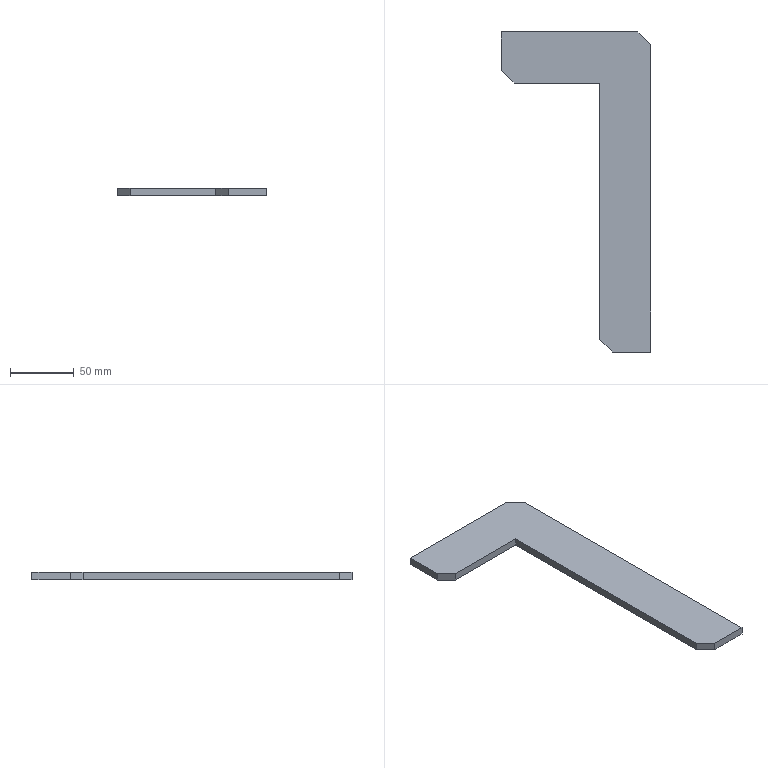Part | STEP file | X77-07102 | 1 solid | 11 faces | box 117 x 250.648 x 6 mm | volume 77736 mm3 | plane 11
STEP:
#1=CARTESIAN_POINT('',(-134.199,-59.214,0.));
#2=VERTEX_POINT('',#1);
#3=CARTESIAN_POINT('',(-241.199,-59.214,0.));
#4=VERTEX_POINT('',#3);
#5=CARTESIAN_POINT('',(-241.199,-59.214,0.));
#6=DIRECTION('',(-1.,0.,0.));
#7=VECTOR('',#6,1000.);
#8=LINE('',#5,#7);
#9=EDGE_CURVE('',#2,#4,#8,.T.);
#10=ORIENTED_EDGE('',*,*,#9,.T.);
#11=CARTESIAN_POINT('',(-241.199,-59.214,6.));
#12=VERTEX_POINT('',#11);
#13=CARTESIAN_POINT('',(-241.199,-59.214,6.));
#14=DIRECTION('',(0.,0.,-1.));
#15=VECTOR('',#14,1000.);
#16=LINE('',#13,#15);
#17=EDGE_CURVE('',#12,#4,#16,.T.);
#18=ORIENTED_EDGE('',*,*,#17,.F.);
#19=CARTESIAN_POINT('',(-134.199,-59.214,6.));
#20=VERTEX_POINT('',#19);
#21=CARTESIAN_POINT('',(-241.199,-59.214,6.));
#22=DIRECTION('',(-1.,0.,0.));
#23=VECTOR('',#22,1000.);
#24=LINE('',#21,#23);
#25=EDGE_CURVE('',#20,#12,#24,.T.);
#26=ORIENTED_EDGE('',*,*,#25,.F.);
#27=CARTESIAN_POINT('',(-134.199,-59.214,6.));
#28=DIRECTION('',(0.,0.,-1.));
#29=VECTOR('',#28,1000.);
#30=LINE('',#27,#29);
#31=EDGE_CURVE('',#20,#2,#30,.T.);
#32=ORIENTED_EDGE('',*,*,#31,.T.);
#33=EDGE_LOOP('',(#10,#18,#26,#32));
#34=FACE_OUTER_BOUND('',#33,.T.);
#35=CARTESIAN_POINT('',(-241.199,-59.214,6.));
#36=DIRECTION('',(0.,-1.,0.));
#37=DIRECTION('',(1.,0.,0.));
#38=AXIS2_PLACEMENT_3D('',#35,#36,#37);
#39=PLANE('',#38);
#40=ADVANCED_FACE('',(#34),#39,.F.);
#41=CARTESIAN_POINT('',(-241.199,-89.214,0.));
#42=VERTEX_POINT('',#41);
#43=CARTESIAN_POINT('',(-241.199,-59.214,0.));
#44=DIRECTION('',(0.,-1.,0.));
#45=VECTOR('',#44,1000.);
#46=LINE('',#43,#45);
#47=EDGE_CURVE('',#4,#42,#46,.T.);
#48=ORIENTED_EDGE('',*,*,#47,.T.);
#49=CARTESIAN_POINT('',(-241.199,-89.214,6.));
#50=VERTEX_POINT('',#49);
#51=CARTESIAN_POINT('',(-241.199,-89.214,6.));
#52=DIRECTION('',(0.,0.,1.));
#53=VECTOR('',#52,1000.);
#54=LINE('',#51,#53);
#55=EDGE_CURVE('',#42,#50,#54,.T.);
#56=ORIENTED_EDGE('',*,*,#55,.T.);
#57=CARTESIAN_POINT('',(-241.199,-59.214,6.));
#58=DIRECTION('',(0.,-1.,0.));
#59=VECTOR('',#58,1000.);
#60=LINE('',#57,#59);
#61=EDGE_CURVE('',#12,#50,#60,.T.);
#62=ORIENTED_EDGE('',*,*,#61,.F.);
#63=ORIENTED_EDGE('',*,*,#17,.T.);
#64=EDGE_LOOP('',(#48,#56,#62,#63));
#65=FACE_OUTER_BOUND('',#64,.T.);
#66=CARTESIAN_POINT('',(-241.199,-59.214,6.));
#67=DIRECTION('',(1.,0.,0.));
#68=DIRECTION('',(0.,1.,0.));
#69=AXIS2_PLACEMENT_3D('',#66,#67,#68);
#70=PLANE('',#69);
#71=ADVANCED_FACE('',(#65),#70,.F.);
#72=CARTESIAN_POINT('',(-231.199,-99.214,6.));
#73=VERTEX_POINT('',#72);
#74=CARTESIAN_POINT('',(-164.199,-99.214,6.));
#75=VERTEX_POINT('',#74);
#76=CARTESIAN_POINT('',(-241.199,-99.214,6.));
#77=DIRECTION('',(1.,0.,0.));
#78=VECTOR('',#77,1000.);
#79=LINE('',#76,#78);
#80=EDGE_CURVE('',#73,#75,#79,.T.);
#81=ORIENTED_EDGE('',*,*,#80,.F.);
#82=CARTESIAN_POINT('',(-231.199,-99.214,0.));
#83=VERTEX_POINT('',#82);
#84=CARTESIAN_POINT('',(-231.199,-99.214,6.));
#85=DIRECTION('',(0.,0.,-1.));
#86=VECTOR('',#85,1000.);
#87=LINE('',#84,#86);
#88=EDGE_CURVE('',#73,#83,#87,.T.);
#89=ORIENTED_EDGE('',*,*,#88,.T.);
#90=CARTESIAN_POINT('',(-164.199,-99.214,0.));
#91=VERTEX_POINT('',#90);
#92=CARTESIAN_POINT('',(-241.199,-99.214,0.));
#93=DIRECTION('',(1.,0.,0.));
#94=VECTOR('',#93,1000.);
#95=LINE('',#92,#94);
#96=EDGE_CURVE('',#83,#91,#95,.T.);
#97=ORIENTED_EDGE('',*,*,#96,.T.);
#98=CARTESIAN_POINT('',(-164.199,-99.214,6.));
#99=DIRECTION('',(0.,0.,-1.));
#100=VECTOR('',#99,1000.);
#101=LINE('',#98,#100);
#102=EDGE_CURVE('',#75,#91,#101,.T.);
#103=ORIENTED_EDGE('',*,*,#102,.F.);
#104=EDGE_LOOP('',(#81,#89,#97,#103));
#105=FACE_OUTER_BOUND('',#104,.T.);
#106=CARTESIAN_POINT('',(-241.199,-99.214,6.));
#107=DIRECTION('',(0.,1.,0.));
#108=DIRECTION('',(0.,0.,1.));
#109=AXIS2_PLACEMENT_3D('',#106,#107,#108);
#110=PLANE('',#109);
#111=ADVANCED_FACE('',(#105),#110,.F.);
#112=CARTESIAN_POINT('',(-164.199,-299.863,0.));
#113=VERTEX_POINT('',#112);
#114=CARTESIAN_POINT('',(-164.199,-99.214,0.));
#115=DIRECTION('',(0.,-1.,0.));
#116=VECTOR('',#115,1000.);
#117=LINE('',#114,#116);
#118=EDGE_CURVE('',#91,#113,#117,.T.);
#119=ORIENTED_EDGE('',*,*,#118,.T.);
#120=CARTESIAN_POINT('',(-164.199,-299.863,6.));
#121=VERTEX_POINT('',#120);
#122=CARTESIAN_POINT('',(-164.199,-299.863,6.));
#123=DIRECTION('',(0.,0.,1.));
#124=VECTOR('',#123,1000.);
#125=LINE('',#122,#124);
#126=EDGE_CURVE('',#113,#121,#125,.T.);
#127=ORIENTED_EDGE('',*,*,#126,.T.);
#128=CARTESIAN_POINT('',(-164.199,-99.214,6.));
#129=DIRECTION('',(0.,-1.,0.));
#130=VECTOR('',#129,1000.);
#131=LINE('',#128,#130);
#132=EDGE_CURVE('',#75,#121,#131,.T.);
#133=ORIENTED_EDGE('',*,*,#132,.F.);
#134=ORIENTED_EDGE('',*,*,#102,.T.);
#135=EDGE_LOOP('',(#119,#127,#133,#134));
#136=FACE_OUTER_BOUND('',#135,.T.);
#137=CARTESIAN_POINT('',(-164.199,-99.214,6.));
#138=DIRECTION('',(1.,0.,0.));
#139=DIRECTION('',(0.,1.,0.));
#140=AXIS2_PLACEMENT_3D('',#137,#138,#139);
#141=PLANE('',#140);
#142=ADVANCED_FACE('',(#136),#141,.F.);
#143=CARTESIAN_POINT('',(-154.199,-309.863,6.));
#144=VERTEX_POINT('',#143);
#145=CARTESIAN_POINT('',(-124.199,-309.863,6.));
#146=VERTEX_POINT('',#145);
#147=CARTESIAN_POINT('',(-164.199,-309.863,6.));
#148=DIRECTION('',(1.,0.,0.));
#149=VECTOR('',#148,1000.);
#150=LINE('',#147,#149);
#151=EDGE_CURVE('',#144,#146,#150,.T.);
#152=ORIENTED_EDGE('',*,*,#151,.F.);
#153=CARTESIAN_POINT('',(-154.199,-309.863,0.));
#154=VERTEX_POINT('',#153);
#155=CARTESIAN_POINT('',(-154.199,-309.863,6.));
#156=DIRECTION('',(0.,0.,-1.));
#157=VECTOR('',#156,1000.);
#158=LINE('',#155,#157);
#159=EDGE_CURVE('',#144,#154,#158,.T.);
#160=ORIENTED_EDGE('',*,*,#159,.T.);
#161=CARTESIAN_POINT('',(-124.199,-309.863,0.));
#162=VERTEX_POINT('',#161);
#163=CARTESIAN_POINT('',(-164.199,-309.863,0.));
#164=DIRECTION('',(1.,0.,0.));
#165=VECTOR('',#164,1000.);
#166=LINE('',#163,#165);
#167=EDGE_CURVE('',#154,#162,#166,.T.);
#168=ORIENTED_EDGE('',*,*,#167,.T.);
#169=CARTESIAN_POINT('',(-124.199,-309.863,6.));
#170=DIRECTION('',(0.,0.,-1.));
#171=VECTOR('',#170,1000.);
#172=LINE('',#169,#171);
#173=EDGE_CURVE('',#146,#162,#172,.T.);
#174=ORIENTED_EDGE('',*,*,#173,.F.);
#175=EDGE_LOOP('',(#152,#160,#168,#174));
#176=FACE_OUTER_BOUND('',#175,.T.);
#177=CARTESIAN_POINT('',(-164.199,-309.863,6.));
#178=DIRECTION('',(0.,1.,0.));
#179=DIRECTION('',(0.,0.,1.));
#180=AXIS2_PLACEMENT_3D('',#177,#178,#179);
#181=PLANE('',#180);
#182=ADVANCED_FACE('',(#176),#181,.F.);
#183=CARTESIAN_POINT('',(-124.199,-69.214,0.));
#184=VERTEX_POINT('',#183);
#185=CARTESIAN_POINT('',(-124.199,-309.863,0.));
#186=DIRECTION('',(0.,1.,0.));
#187=VECTOR('',#186,1000.);
#188=LINE('',#185,#187);
#189=EDGE_CURVE('',#162,#184,#188,.T.);
#190=ORIENTED_EDGE('',*,*,#189,.T.);
#191=CARTESIAN_POINT('',(-124.199,-69.214,6.));
#192=VERTEX_POINT('',#191);
#193=CARTESIAN_POINT('',(-124.199,-69.214,6.));
#194=DIRECTION('',(0.,0.,-1.));
#195=VECTOR('',#194,1000.);
#196=LINE('',#193,#195);
#197=EDGE_CURVE('',#192,#184,#196,.T.);
#198=ORIENTED_EDGE('',*,*,#197,.F.);
#199=CARTESIAN_POINT('',(-124.199,-309.863,6.));
#200=DIRECTION('',(0.,1.,0.));
#201=VECTOR('',#200,1000.);
#202=LINE('',#199,#201);
#203=EDGE_CURVE('',#146,#192,#202,.T.);
#204=ORIENTED_EDGE('',*,*,#203,.F.);
#205=ORIENTED_EDGE('',*,*,#173,.T.);
#206=EDGE_LOOP('',(#190,#198,#204,#205));
#207=FACE_OUTER_BOUND('',#206,.T.);
#208=CARTESIAN_POINT('',(-124.199,-309.863,6.));
#209=DIRECTION('',(-1.,0.,0.));
#210=DIRECTION('',(0.,-1.,0.));
#211=AXIS2_PLACEMENT_3D('',#208,#209,#210);
#212=PLANE('',#211);
#213=ADVANCED_FACE('',(#207),#212,.F.);
#214=CARTESIAN_POINT('',(-134.199,-59.214,0.));
#215=DIRECTION('',(-0.7071,0.7071,0.));
#216=VECTOR('',#215,1000.);
#217=LINE('',#214,#216);
#218=EDGE_CURVE('',#184,#2,#217,.T.);
#219=ORIENTED_EDGE('',*,*,#218,.T.);
#220=ORIENTED_EDGE('',*,*,#31,.F.);
#221=CARTESIAN_POINT('',(-134.199,-59.214,6.));
#222=DIRECTION('',(-0.7071,0.7071,0.));
#223=VECTOR('',#222,1000.);
#224=LINE('',#221,#223);
#225=EDGE_CURVE('',#192,#20,#224,.T.);
#226=ORIENTED_EDGE('',*,*,#225,.F.);
#227=ORIENTED_EDGE('',*,*,#197,.T.);
#228=EDGE_LOOP('',(#219,#220,#226,#227));
#229=FACE_OUTER_BOUND('',#228,.T.);
#230=CARTESIAN_POINT('',(-134.199,-59.214,6.));
#231=DIRECTION('',(-0.7071,-0.7071,0.));
#232=DIRECTION('',(0.7071,-0.7071,0.));
#233=AXIS2_PLACEMENT_3D('',#230,#231,#232);
#234=PLANE('',#233);
#235=ADVANCED_FACE('',(#229),#234,.F.);
#236=ORIENTED_EDGE('',*,*,#132,.T.);
#237=CARTESIAN_POINT('',(-264.523,-199.538,6.));
#238=DIRECTION('',(0.7071,-0.7071,0.));
#239=VECTOR('',#238,1000.);
#240=LINE('',#237,#239);
#241=EDGE_CURVE('',#121,#144,#240,.T.);
#242=ORIENTED_EDGE('',*,*,#241,.T.);
#243=ORIENTED_EDGE('',*,*,#151,.T.);
#244=ORIENTED_EDGE('',*,*,#203,.T.);
#245=ORIENTED_EDGE('',*,*,#225,.T.);
#246=ORIENTED_EDGE('',*,*,#25,.T.);
#247=ORIENTED_EDGE('',*,*,#61,.T.);
#248=CARTESIAN_POINT('',(-197.699,-132.714,6.));
#249=DIRECTION('',(0.7071,-0.7071,0.));
#250=VECTOR('',#249,1000.);
#251=LINE('',#248,#250);
#252=EDGE_CURVE('',#50,#73,#251,.T.);
#253=ORIENTED_EDGE('',*,*,#252,.T.);
#254=ORIENTED_EDGE('',*,*,#80,.T.);
#255=EDGE_LOOP('',(#236,#242,#243,#244,#245,#246,#247,#253,#254));
#256=FACE_OUTER_BOUND('',#255,.T.);
#257=CARTESIAN_POINT('',(-124.199,-59.214,6.));
#258=DIRECTION('',(0.,0.,1.));
#259=DIRECTION('',(1.,0.,0.));
#260=AXIS2_PLACEMENT_3D('',#257,#258,#259);
#261=PLANE('',#260);
#262=ADVANCED_FACE('',(#256),#261,.T.);
#263=ORIENTED_EDGE('',*,*,#167,.F.);
#264=CARTESIAN_POINT('',(-154.199,-309.863,0.));
#265=DIRECTION('',(-0.7071,0.7071,0.));
#266=VECTOR('',#265,1000.);
#267=LINE('',#264,#266);
#268=EDGE_CURVE('',#154,#113,#267,.T.);
#269=ORIENTED_EDGE('',*,*,#268,.T.);
#270=ORIENTED_EDGE('',*,*,#118,.F.);
#271=ORIENTED_EDGE('',*,*,#96,.F.);
#272=CARTESIAN_POINT('',(-231.199,-99.214,0.));
#273=DIRECTION('',(-0.7071,0.7071,0.));
#274=VECTOR('',#273,1000.);
#275=LINE('',#272,#274);
#276=EDGE_CURVE('',#83,#42,#275,.T.);
#277=ORIENTED_EDGE('',*,*,#276,.T.);
#278=ORIENTED_EDGE('',*,*,#47,.F.);
#279=ORIENTED_EDGE('',*,*,#9,.F.);
#280=ORIENTED_EDGE('',*,*,#218,.F.);
#281=ORIENTED_EDGE('',*,*,#189,.F.);
#282=EDGE_LOOP('',(#263,#269,#270,#271,#277,#278,#279,#280,#281));
#283=FACE_OUTER_BOUND('',#282,.T.);
#284=CARTESIAN_POINT('',(-124.199,-59.214,0.));
#285=DIRECTION('',(0.,0.,1.));
#286=DIRECTION('',(1.,0.,0.));
#287=AXIS2_PLACEMENT_3D('',#284,#285,#286);
#288=PLANE('',#287);
#289=ADVANCED_FACE('',(#283),#288,.F.);
#290=ORIENTED_EDGE('',*,*,#241,.F.);
#291=ORIENTED_EDGE('',*,*,#126,.F.);
#292=ORIENTED_EDGE('',*,*,#268,.F.);
#293=ORIENTED_EDGE('',*,*,#159,.F.);
#294=EDGE_LOOP('',(#290,#291,#292,#293));
#295=FACE_OUTER_BOUND('',#294,.T.);
#296=CARTESIAN_POINT('',(-154.199,-309.863,6.));
#297=DIRECTION('',(0.7071,0.7071,0.));
#298=DIRECTION('',(-0.7071,0.7071,0.));
#299=AXIS2_PLACEMENT_3D('',#296,#297,#298);
#300=PLANE('',#299);
#301=ADVANCED_FACE('',(#295),#300,.F.);
#302=ORIENTED_EDGE('',*,*,#252,.F.);
#303=ORIENTED_EDGE('',*,*,#55,.F.);
#304=ORIENTED_EDGE('',*,*,#276,.F.);
#305=ORIENTED_EDGE('',*,*,#88,.F.);
#306=EDGE_LOOP('',(#302,#303,#304,#305));
#307=FACE_OUTER_BOUND('',#306,.T.);
#308=CARTESIAN_POINT('',(-231.199,-99.214,6.));
#309=DIRECTION('',(0.7071,0.7071,0.));
#310=DIRECTION('',(-0.7071,0.7071,0.));
#311=AXIS2_PLACEMENT_3D('',#308,#309,#310);
#312=PLANE('',#311);
#313=ADVANCED_FACE('',(#307),#312,.F.);
#314=CLOSED_SHELL('',(#40,#71,#111,#142,#182,#213,#235,#262,#289,#301,#313));
#315=MANIFOLD_SOLID_BREP('',#314);
#316=CARTESIAN_POINT('',(0.,0.,0.));
#317=DIRECTION('',(0.,0.,1.));
#318=DIRECTION('',(1.,0.,0.));
#319=AXIS2_PLACEMENT_3D('',#316,#317,#318);
#320=(LENGTH_UNIT()NAMED_UNIT(*)SI_UNIT(.MILLI.,.METRE.));
#321=UNCERTAINTY_MEASURE_WITH_UNIT(LENGTH_MEASURE(0.00001),#320,'','');
#322=(NAMED_UNIT(*)PLANE_ANGLE_UNIT()SI_UNIT($,.RADIAN.));
#323=(NAMED_UNIT(*)SI_UNIT($,.STERADIAN.)SOLID_ANGLE_UNIT());
#324=(GEOMETRIC_REPRESENTATION_CONTEXT(3)GLOBAL_UNCERTAINTY_ASSIGNED_CONTEXT((#321))GLOBAL_UNIT_ASSIGNED_CONTEXT((#320,#322,#323))REPRESENTATION_CONTEXT('',''));
#325=ADVANCED_BREP_SHAPE_REPRESENTATION('',(#315,#319),#324);